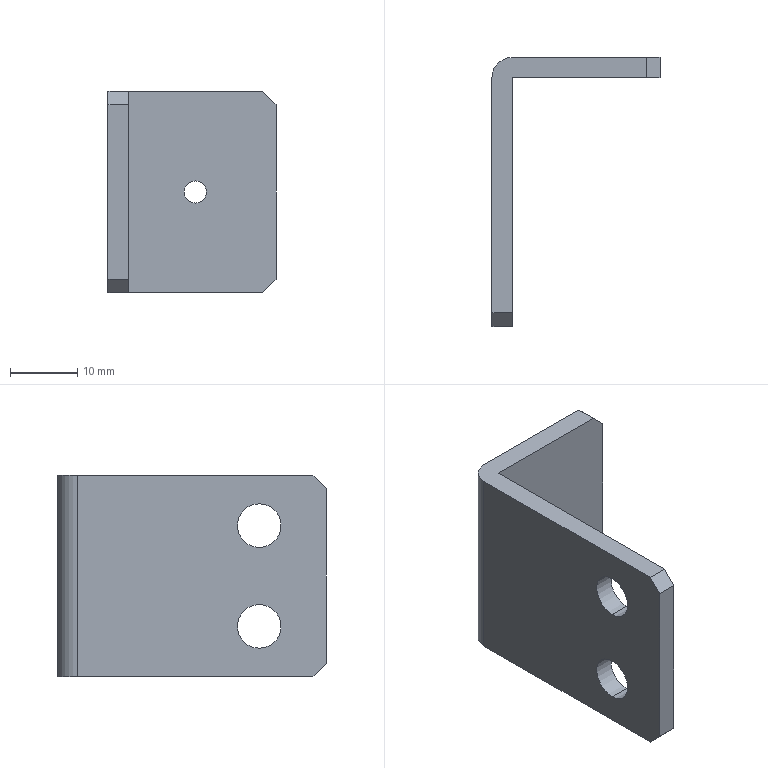Part | STEP file | 0228_210_Bracket | 1 solid | 19 faces | box 25 x 40 x 30 mm | volume 5273 mm3 | plane 12 | cylinder 7 | commonest cylinder face diameters 6.5 x4 3.3 x2 6 x1
STEP:
#1=CARTESIAN_POINT('',(0.,0.,0.));
#2=DIRECTION('',(0.,0.,1.));
#3=DIRECTION('',(1.,0.,0.));
#4=AXIS2_PLACEMENT_3D('',#1,#2,#3);
#5=CARTESIAN_POINT('',(13.,-3.,1.65));
#6=VERTEX_POINT('',#5);
#7=CARTESIAN_POINT('',(13.,0.,1.65));
#8=VERTEX_POINT('',#7);
#9=CARTESIAN_POINT('',(13.,0.,1.65));
#10=DIRECTION('',(0.,1.,0.));
#11=VECTOR('',#10,1.);
#12=LINE('',#9,#11);
#13=CARTESIAN_POINT('',(13.,0.,0.));
#14=DIRECTION('',(0.,1.,0.));
#15=DIRECTION('',(0.,0.,1.));
#16=AXIS2_PLACEMENT_3D('',#13,#14,#15);
#17=CYLINDRICAL_SURFACE('',#16,1.65);
#18=CARTESIAN_POINT('',(6.283,0.));
#19=DIRECTION('',(0.,1.));
#20=VECTOR('',#19,1.);
#21=LINE('',#18,#20);
#22=(GEOMETRIC_REPRESENTATION_CONTEXT(2)PARAMETRIC_REPRESENTATION_CONTEXT()REPRESENTATION_CONTEXT('',''));
#23=DEFINITIONAL_REPRESENTATION('',(#21),#22);
#24=PCURVE('',#17,#23);
#25=CARTESIAN_POINT('',(13.,0.,0.));
#26=DIRECTION('',(0.,1.,0.));
#27=DIRECTION('',(0.,0.,1.));
#28=AXIS2_PLACEMENT_3D('',#25,#26,#27);
#29=CYLINDRICAL_SURFACE('',#28,1.65);
#30=CARTESIAN_POINT('',(0.,0.));
#31=DIRECTION('',(0.,1.));
#32=VECTOR('',#31,1.);
#33=LINE('',#30,#32);
#34=(GEOMETRIC_REPRESENTATION_CONTEXT(2)PARAMETRIC_REPRESENTATION_CONTEXT()REPRESENTATION_CONTEXT('',''));
#35=DEFINITIONAL_REPRESENTATION('',(#33),#34);
#36=PCURVE('',#29,#35);
#37=SURFACE_CURVE('',#12,(#24,#36),.PCURVE_S1.);
#38=EDGE_CURVE('',#6,#8,#37,.T.);
#39=ORIENTED_EDGE('',*,*,#38,.T.);
#40=CARTESIAN_POINT('',(13.,0.,-1.65));
#41=VERTEX_POINT('',#40);
#42=CARTESIAN_POINT('',(13.,0.,0.));
#43=DIRECTION('',(0.,1.,0.));
#44=DIRECTION('',(0.,0.,1.));
#45=AXIS2_PLACEMENT_3D('',#42,#43,#44);
#46=CIRCLE('',#45,1.65);
#47=CARTESIAN_POINT('',(0.,0.));
#48=DIRECTION('',(1.,0.));
#49=VECTOR('',#48,1.);
#50=LINE('',#47,#49);
#51=(GEOMETRIC_REPRESENTATION_CONTEXT(2)PARAMETRIC_REPRESENTATION_CONTEXT()REPRESENTATION_CONTEXT('',''));
#52=DEFINITIONAL_REPRESENTATION('',(#50),#51);
#53=PCURVE('',#17,#52);
#54=CARTESIAN_POINT('',(25.,0.,15.));
#55=DIRECTION('',(0.,-1.,0.));
#56=DIRECTION('',(1.,0.,0.));
#57=AXIS2_PLACEMENT_3D('',#54,#55,#56);
#58=PLANE('',#57);
#59=CARTESIAN_POINT('',(-12.,-13.35));
#60=CARTESIAN_POINT('',(-9.142,-13.35));
#61=CARTESIAN_POINT('',(-10.571,-15.825));
#62=CARTESIAN_POINT('',(-12.,-18.3));
#63=CARTESIAN_POINT('',(-13.429,-15.825));
#64=CARTESIAN_POINT('',(-14.858,-13.35));
#65=CARTESIAN_POINT('',(-12.,-13.35));
#66=(BOUNDED_CURVE()B_SPLINE_CURVE(2,(#59,#60,#61,#62,#63,#64,#65),.UNSPECIFIED.,.T.,.F.)B_SPLINE_CURVE_WITH_KNOTS((1,2,2,2,2,1),(-2.094,0.,2.094,4.189,6.283,8.378),.UNSPECIFIED.)CURVE()GEOMETRIC_REPRESENTATION_ITEM()RATIONAL_B_SPLINE_CURVE((1.,0.5,1.,0.5,1.,0.5,1.))REPRESENTATION_ITEM(''));
#67=(GEOMETRIC_REPRESENTATION_CONTEXT(2)PARAMETRIC_REPRESENTATION_CONTEXT()REPRESENTATION_CONTEXT('',''));
#68=DEFINITIONAL_REPRESENTATION('',(#66),#67);
#69=PCURVE('',#58,#68);
#70=SURFACE_CURVE('',#46,(#53,#69),.PCURVE_S1.);
#71=EDGE_CURVE('',#41,#8,#70,.T.);
#72=ORIENTED_EDGE('',*,*,#71,.F.);
#73=CARTESIAN_POINT('',(13.,-3.,-1.65));
#74=VERTEX_POINT('',#73);
#75=CARTESIAN_POINT('',(13.,0.,-1.65));
#76=DIRECTION('',(0.,1.,0.));
#77=VECTOR('',#76,1.);
#78=LINE('',#75,#77);
#79=CARTESIAN_POINT('',(3.142,0.));
#80=DIRECTION('',(0.,1.));
#81=VECTOR('',#80,1.);
#82=LINE('',#79,#81);
#83=(GEOMETRIC_REPRESENTATION_CONTEXT(2)PARAMETRIC_REPRESENTATION_CONTEXT()REPRESENTATION_CONTEXT('',''));
#84=DEFINITIONAL_REPRESENTATION('',(#82),#83);
#85=PCURVE('',#17,#84);
#86=CARTESIAN_POINT('',(3.142,0.));
#87=DIRECTION('',(0.,1.));
#88=VECTOR('',#87,1.);
#89=LINE('',#86,#88);
#90=(GEOMETRIC_REPRESENTATION_CONTEXT(2)PARAMETRIC_REPRESENTATION_CONTEXT()REPRESENTATION_CONTEXT('',''));
#91=DEFINITIONAL_REPRESENTATION('',(#89),#90);
#92=PCURVE('',#29,#91);
#93=SURFACE_CURVE('',#78,(#85,#92),.PCURVE_S1.);
#94=EDGE_CURVE('',#74,#41,#93,.T.);
#95=ORIENTED_EDGE('',*,*,#94,.F.);
#96=CARTESIAN_POINT('',(13.,-3.,0.));
#97=DIRECTION('',(0.,1.,0.));
#98=DIRECTION('',(-1.,0.,0.));
#99=AXIS2_PLACEMENT_3D('',#96,#97,#98);
#100=CIRCLE('',#99,1.65);
#101=CARTESIAN_POINT('',(-1.571,-3.));
#102=DIRECTION('',(1.,0.));
#103=VECTOR('',#102,1.);
#104=LINE('',#101,#103);
#105=(GEOMETRIC_REPRESENTATION_CONTEXT(2)PARAMETRIC_REPRESENTATION_CONTEXT()REPRESENTATION_CONTEXT('',''));
#106=DEFINITIONAL_REPRESENTATION('',(#104),#105);
#107=PCURVE('',#17,#106);
#108=CARTESIAN_POINT('',(25.,-3.,15.));
#109=DIRECTION('',(0.,1.,0.));
#110=DIRECTION('',(-1.,0.,0.));
#111=AXIS2_PLACEMENT_3D('',#108,#109,#110);
#112=PLANE('',#111);
#113=CARTESIAN_POINT('',(12.,-15.));
#114=DIRECTION('',(1.,0.));
#115=AXIS2_PLACEMENT_2D('',#113,#114);
#116=CIRCLE('',#115,1.65);
#117=(GEOMETRIC_REPRESENTATION_CONTEXT(2)PARAMETRIC_REPRESENTATION_CONTEXT()REPRESENTATION_CONTEXT('',''));
#118=DEFINITIONAL_REPRESENTATION('',(#116),#117);
#119=PCURVE('',#112,#118);
#120=SURFACE_CURVE('',#100,(#107,#119),.PCURVE_S1.);
#121=EDGE_CURVE('',#74,#6,#120,.T.);
#122=ORIENTED_EDGE('',*,*,#121,.T.);
#123=EDGE_LOOP('',(#39,#72,#95,#122));
#124=FACE_BOUND('',#123,.F.);
#125=ADVANCED_FACE('',(#124),#17,.F.);
#126=CARTESIAN_POINT('',(0.,-30.,4.25));
#127=VERTEX_POINT('',#126);
#128=CARTESIAN_POINT('',(3.,-30.,4.25));
#129=VERTEX_POINT('',#128);
#130=CARTESIAN_POINT('',(3.,-30.,4.25));
#131=DIRECTION('',(1.,0.,0.));
#132=VECTOR('',#131,1.);
#133=LINE('',#130,#132);
#134=CARTESIAN_POINT('',(3.,-30.,7.5));
#135=DIRECTION('',(1.,0.,0.));
#136=DIRECTION('',(0.,0.,-1.));
#137=AXIS2_PLACEMENT_3D('',#134,#135,#136);
#138=CYLINDRICAL_SURFACE('',#137,3.25);
#139=CARTESIAN_POINT('',(6.283,0.));
#140=DIRECTION('',(0.,1.));
#141=VECTOR('',#140,1.);
#142=LINE('',#139,#141);
#143=(GEOMETRIC_REPRESENTATION_CONTEXT(2)PARAMETRIC_REPRESENTATION_CONTEXT()REPRESENTATION_CONTEXT('',''));
#144=DEFINITIONAL_REPRESENTATION('',(#142),#143);
#145=PCURVE('',#138,#144);
#146=CARTESIAN_POINT('',(3.,-30.,7.5));
#147=DIRECTION('',(1.,0.,0.));
#148=DIRECTION('',(0.,0.,-1.));
#149=AXIS2_PLACEMENT_3D('',#146,#147,#148);
#150=CYLINDRICAL_SURFACE('',#149,3.25);
#151=CARTESIAN_POINT('',(0.,0.));
#152=DIRECTION('',(0.,1.));
#153=VECTOR('',#152,1.);
#154=LINE('',#151,#153);
#155=(GEOMETRIC_REPRESENTATION_CONTEXT(2)PARAMETRIC_REPRESENTATION_CONTEXT()REPRESENTATION_CONTEXT('',''));
#156=DEFINITIONAL_REPRESENTATION('',(#154),#155);
#157=PCURVE('',#150,#156);
#158=SURFACE_CURVE('',#133,(#145,#157),.PCURVE_S1.);
#159=EDGE_CURVE('',#127,#129,#158,.T.);
#160=ORIENTED_EDGE('',*,*,#159,.T.);
#161=CARTESIAN_POINT('',(3.,-30.,10.75));
#162=VERTEX_POINT('',#161);
#163=CARTESIAN_POINT('',(3.,-30.,7.5));
#164=DIRECTION('',(1.,0.,0.));
#165=DIRECTION('',(0.,0.,-1.));
#166=AXIS2_PLACEMENT_3D('',#163,#164,#165);
#167=CIRCLE('',#166,3.25);
#168=CARTESIAN_POINT('',(0.,0.));
#169=DIRECTION('',(1.,0.));
#170=VECTOR('',#169,1.);
#171=LINE('',#168,#170);
#172=(GEOMETRIC_REPRESENTATION_CONTEXT(2)PARAMETRIC_REPRESENTATION_CONTEXT()REPRESENTATION_CONTEXT('',''));
#173=DEFINITIONAL_REPRESENTATION('',(#171),#172);
#174=PCURVE('',#138,#173);
#175=CARTESIAN_POINT('',(3.,-3.,15.));
#176=DIRECTION('',(-1.,0.,0.));
#177=DIRECTION('',(0.,-1.,0.));
#178=AXIS2_PLACEMENT_3D('',#175,#176,#177);
#179=PLANE('',#178);
#180=CARTESIAN_POINT('',(27.,-10.75));
#181=CARTESIAN_POINT('',(21.371,-10.75));
#182=CARTESIAN_POINT('',(24.185,-5.875));
#183=CARTESIAN_POINT('',(27.,-1.));
#184=CARTESIAN_POINT('',(29.815,-5.875));
#185=CARTESIAN_POINT('',(32.629,-10.75));
#186=CARTESIAN_POINT('',(27.,-10.75));
#187=(BOUNDED_CURVE()B_SPLINE_CURVE(2,(#180,#181,#182,#183,#184,#185,#186),.UNSPECIFIED.,.T.,.F.)B_SPLINE_CURVE_WITH_KNOTS((1,2,2,2,2,1),(-2.094,0.,2.094,4.189,6.283,8.378),.UNSPECIFIED.)CURVE()GEOMETRIC_REPRESENTATION_ITEM()RATIONAL_B_SPLINE_CURVE((1.,0.5,1.,0.5,1.,0.5,1.))REPRESENTATION_ITEM(''));
#188=(GEOMETRIC_REPRESENTATION_CONTEXT(2)PARAMETRIC_REPRESENTATION_CONTEXT()REPRESENTATION_CONTEXT('',''));
#189=DEFINITIONAL_REPRESENTATION('',(#187),#188);
#190=PCURVE('',#179,#189);
#191=SURFACE_CURVE('',#167,(#174,#190),.PCURVE_S1.);
#192=EDGE_CURVE('',#162,#129,#191,.T.);
#193=ORIENTED_EDGE('',*,*,#192,.F.);
#194=CARTESIAN_POINT('',(0.,-30.,10.75));
#195=VERTEX_POINT('',#194);
#196=CARTESIAN_POINT('',(3.,-30.,10.75));
#197=DIRECTION('',(1.,0.,0.));
#198=VECTOR('',#197,1.);
#199=LINE('',#196,#198);
#200=CARTESIAN_POINT('',(3.142,0.));
#201=DIRECTION('',(0.,1.));
#202=VECTOR('',#201,1.);
#203=LINE('',#200,#202);
#204=(GEOMETRIC_REPRESENTATION_CONTEXT(2)PARAMETRIC_REPRESENTATION_CONTEXT()REPRESENTATION_CONTEXT('',''));
#205=DEFINITIONAL_REPRESENTATION('',(#203),#204);
#206=PCURVE('',#138,#205);
#207=CARTESIAN_POINT('',(3.142,0.));
#208=DIRECTION('',(0.,1.));
#209=VECTOR('',#208,1.);
#210=LINE('',#207,#209);
#211=(GEOMETRIC_REPRESENTATION_CONTEXT(2)PARAMETRIC_REPRESENTATION_CONTEXT()REPRESENTATION_CONTEXT('',''));
#212=DEFINITIONAL_REPRESENTATION('',(#210),#211);
#213=PCURVE('',#150,#212);
#214=SURFACE_CURVE('',#199,(#206,#213),.PCURVE_S1.);
#215=EDGE_CURVE('',#195,#162,#214,.T.);
#216=ORIENTED_EDGE('',*,*,#215,.F.);
#217=CARTESIAN_POINT('',(0.,-30.,7.5));
#218=DIRECTION('',(1.,0.,0.));
#219=DIRECTION('',(0.,0.,-1.));
#220=AXIS2_PLACEMENT_3D('',#217,#218,#219);
#221=CIRCLE('',#220,3.25);
#222=CARTESIAN_POINT('',(0.,-3.));
#223=DIRECTION('',(1.,0.));
#224=VECTOR('',#223,1.);
#225=LINE('',#222,#224);
#226=(GEOMETRIC_REPRESENTATION_CONTEXT(2)PARAMETRIC_REPRESENTATION_CONTEXT()REPRESENTATION_CONTEXT('',''));
#227=DEFINITIONAL_REPRESENTATION('',(#225),#226);
#228=PCURVE('',#138,#227);
#229=CARTESIAN_POINT('',(0.,0.,15.));
#230=DIRECTION('',(1.,0.,0.));
#231=DIRECTION('',(0.,1.,0.));
#232=AXIS2_PLACEMENT_3D('',#229,#230,#231);
#233=PLANE('',#232);
#234=CARTESIAN_POINT('',(-30.,-7.5));
#235=DIRECTION('',(0.,-1.));
#236=AXIS2_PLACEMENT_2D('',#234,#235);
#237=CIRCLE('',#236,3.25);
#238=(GEOMETRIC_REPRESENTATION_CONTEXT(2)PARAMETRIC_REPRESENTATION_CONTEXT()REPRESENTATION_CONTEXT('',''));
#239=DEFINITIONAL_REPRESENTATION('',(#237),#238);
#240=PCURVE('',#233,#239);
#241=SURFACE_CURVE('',#221,(#228,#240),.PCURVE_S1.);
#242=EDGE_CURVE('',#195,#127,#241,.T.);
#243=ORIENTED_EDGE('',*,*,#242,.T.);
#244=EDGE_LOOP('',(#160,#193,#216,#243));
#245=FACE_BOUND('',#244,.F.);
#246=ADVANCED_FACE('',(#245),#138,.F.);
#247=CARTESIAN_POINT('',(0.,-30.,-10.75));
#248=VERTEX_POINT('',#247);
#249=CARTESIAN_POINT('',(3.,-30.,-10.75));
#250=VERTEX_POINT('',#249);
#251=CARTESIAN_POINT('',(3.,-30.,-10.75));
#252=DIRECTION('',(1.,0.,0.));
#253=VECTOR('',#252,1.);
#254=LINE('',#251,#253);
#255=CARTESIAN_POINT('',(3.,-30.,-7.5));
#256=DIRECTION('',(1.,0.,0.));
#257=DIRECTION('',(0.,0.,-1.));
#258=AXIS2_PLACEMENT_3D('',#255,#256,#257);
#259=CYLINDRICAL_SURFACE('',#258,3.25);
#260=CARTESIAN_POINT('',(6.283,0.));
#261=DIRECTION('',(0.,1.));
#262=VECTOR('',#261,1.);
#263=LINE('',#260,#262);
#264=(GEOMETRIC_REPRESENTATION_CONTEXT(2)PARAMETRIC_REPRESENTATION_CONTEXT()REPRESENTATION_CONTEXT('',''));
#265=DEFINITIONAL_REPRESENTATION('',(#263),#264);
#266=PCURVE('',#259,#265);
#267=CARTESIAN_POINT('',(3.,-30.,-7.5));
#268=DIRECTION('',(1.,0.,0.));
#269=DIRECTION('',(0.,0.,-1.));
#270=AXIS2_PLACEMENT_3D('',#267,#268,#269);
#271=CYLINDRICAL_SURFACE('',#270,3.25);
#272=CARTESIAN_POINT('',(0.,0.));
#273=DIRECTION('',(0.,1.));
#274=VECTOR('',#273,1.);
#275=LINE('',#272,#274);
#276=(GEOMETRIC_REPRESENTATION_CONTEXT(2)PARAMETRIC_REPRESENTATION_CONTEXT()REPRESENTATION_CONTEXT('',''));
#277=DEFINITIONAL_REPRESENTATION('',(#275),#276);
#278=PCURVE('',#271,#277);
#279=SURFACE_CURVE('',#254,(#266,#278),.PCURVE_S1.);
#280=EDGE_CURVE('',#248,#250,#279,.T.);
#281=ORIENTED_EDGE('',*,*,#280,.T.);
#282=CARTESIAN_POINT('',(3.,-30.,-4.25));
#283=VERTEX_POINT('',#282);
#284=CARTESIAN_POINT('',(3.,-30.,-7.5));
#285=DIRECTION('',(1.,0.,0.));
#286=DIRECTION('',(0.,0.,-1.));
#287=AXIS2_PLACEMENT_3D('',#284,#285,#286);
#288=CIRCLE('',#287,3.25);
#289=CARTESIAN_POINT('',(0.,0.));
#290=DIRECTION('',(1.,0.));
#291=VECTOR('',#290,1.);
#292=LINE('',#289,#291);
#293=(GEOMETRIC_REPRESENTATION_CONTEXT(2)PARAMETRIC_REPRESENTATION_CONTEXT()REPRESENTATION_CONTEXT('',''));
#294=DEFINITIONAL_REPRESENTATION('',(#292),#293);
#295=PCURVE('',#259,#294);
#296=CARTESIAN_POINT('',(27.,-25.75));
#297=CARTESIAN_POINT('',(21.371,-25.75));
#298=CARTESIAN_POINT('',(24.185,-20.875));
#299=CARTESIAN_POINT('',(27.,-16.));
#300=CARTESIAN_POINT('',(29.815,-20.875));
#301=CARTESIAN_POINT('',(32.629,-25.75));
#302=CARTESIAN_POINT('',(27.,-25.75));
#303=(BOUNDED_CURVE()B_SPLINE_CURVE(2,(#296,#297,#298,#299,#300,#301,#302),.UNSPECIFIED.,.T.,.F.)B_SPLINE_CURVE_WITH_KNOTS((1,2,2,2,2,1),(-2.094,0.,2.094,4.189,6.283,8.378),.UNSPECIFIED.)CURVE()GEOMETRIC_REPRESENTATION_ITEM()RATIONAL_B_SPLINE_CURVE((1.,0.5,1.,0.5,1.,0.5,1.))REPRESENTATION_ITEM(''));
#304=(GEOMETRIC_REPRESENTATION_CONTEXT(2)PARAMETRIC_REPRESENTATION_CONTEXT()REPRESENTATION_CONTEXT('',''));
#305=DEFINITIONAL_REPRESENTATION('',(#303),#304);
#306=PCURVE('',#179,#305);
#307=SURFACE_CURVE('',#288,(#295,#306),.PCURVE_S1.);
#308=EDGE_CURVE('',#283,#250,#307,.T.);
#309=ORIENTED_EDGE('',*,*,#308,.F.);
#310=CARTESIAN_POINT('',(0.,-30.,-4.25));
#311=VERTEX_POINT('',#310);
#312=CARTESIAN_POINT('',(3.,-30.,-4.25));
#313=DIRECTION('',(1.,0.,0.));
#314=VECTOR('',#313,1.);
#315=LINE('',#312,#314);
#316=CARTESIAN_POINT('',(3.142,0.));
#317=DIRECTION('',(0.,1.));
#318=VECTOR('',#317,1.);
#319=LINE('',#316,#318);
#320=(GEOMETRIC_REPRESENTATION_CONTEXT(2)PARAMETRIC_REPRESENTATION_CONTEXT()REPRESENTATION_CONTEXT('',''));
#321=DEFINITIONAL_REPRESENTATION('',(#319),#320);
#322=PCURVE('',#259,#321);
#323=CARTESIAN_POINT('',(3.142,0.));
#324=DIRECTION('',(0.,1.));
#325=VECTOR('',#324,1.);
#326=LINE('',#323,#325);
#327=(GEOMETRIC_REPRESENTATION_CONTEXT(2)PARAMETRIC_REPRESENTATION_CONTEXT()REPRESENTATION_CONTEXT('',''));
#328=DEFINITIONAL_REPRESENTATION('',(#326),#327);
#329=PCURVE('',#271,#328);
#330=SURFACE_CURVE('',#315,(#322,#329),.PCURVE_S1.);
#331=EDGE_CURVE('',#311,#283,#330,.T.);
#332=ORIENTED_EDGE('',*,*,#331,.F.);
#333=CARTESIAN_POINT('',(0.,-30.,-7.5));
#334=DIRECTION('',(1.,0.,0.));
#335=DIRECTION('',(0.,0.,-1.));
#336=AXIS2_PLACEMENT_3D('',#333,#334,#335);
#337=CIRCLE('',#336,3.25);
#338=CARTESIAN_POINT('',(0.,-3.));
#339=DIRECTION('',(1.,0.));
#340=VECTOR('',#339,1.);
#341=LINE('',#338,#340);
#342=(GEOMETRIC_REPRESENTATION_CONTEXT(2)PARAMETRIC_REPRESENTATION_CONTEXT()REPRESENTATION_CONTEXT('',''));
#343=DEFINITIONAL_REPRESENTATION('',(#341),#342);
#344=PCURVE('',#259,#343);
#345=CARTESIAN_POINT('',(-30.,-22.5));
#346=DIRECTION('',(0.,-1.));
#347=AXIS2_PLACEMENT_2D('',#345,#346);
#348=CIRCLE('',#347,3.25);
#349=(GEOMETRIC_REPRESENTATION_CONTEXT(2)PARAMETRIC_REPRESENTATION_CONTEXT()REPRESENTATION_CONTEXT('',''));
#350=DEFINITIONAL_REPRESENTATION('',(#348),#349);
#351=PCURVE('',#233,#350);
#352=SURFACE_CURVE('',#337,(#344,#351),.PCURVE_S1.);
#353=EDGE_CURVE('',#311,#248,#352,.T.);
#354=ORIENTED_EDGE('',*,*,#353,.T.);
#355=EDGE_LOOP('',(#281,#309,#332,#354));
#356=FACE_BOUND('',#355,.F.);
#357=ADVANCED_FACE('',(#356),#259,.F.);
#358=CARTESIAN_POINT('',(25.,-3.,13.));
#359=VERTEX_POINT('',#358);
#360=CARTESIAN_POINT('',(25.,-3.,-13.));
#361=VERTEX_POINT('',#360);
#362=CARTESIAN_POINT('',(25.,-3.,15.));
#363=DIRECTION('',(0.,0.,-1.));
#364=VECTOR('',#363,1.);
#365=LINE('',#362,#364);
#366=CARTESIAN_POINT('',(25.,0.,15.));
#367=DIRECTION('',(-1.,0.,0.));
#368=DIRECTION('',(0.,0.,1.));
#369=AXIS2_PLACEMENT_3D('',#366,#367,#368);
#370=PLANE('',#369);
#371=CARTESIAN_POINT('',(0.,-3.));
#372=DIRECTION('',(-1.,0.));
#373=VECTOR('',#372,1.);
#374=LINE('',#371,#373);
#375=(GEOMETRIC_REPRESENTATION_CONTEXT(2)PARAMETRIC_REPRESENTATION_CONTEXT()REPRESENTATION_CONTEXT('',''));
#376=DEFINITIONAL_REPRESENTATION('',(#374),#375);
#377=PCURVE('',#370,#376);
#378=CARTESIAN_POINT('',(0.,0.));
#379=DIRECTION('',(0.,-1.));
#380=VECTOR('',#379,1.);
#381=LINE('',#378,#380);
#382=(GEOMETRIC_REPRESENTATION_CONTEXT(2)PARAMETRIC_REPRESENTATION_CONTEXT()REPRESENTATION_CONTEXT('',''));
#383=DEFINITIONAL_REPRESENTATION('',(#381),#382);
#384=PCURVE('',#112,#383);
#385=SURFACE_CURVE('',#365,(#377,#384),.PCURVE_S1.);
#386=EDGE_CURVE('',#359,#361,#385,.T.);
#387=ORIENTED_EDGE('',*,*,#386,.T.);
#388=CARTESIAN_POINT('',(25.,0.,-13.));
#389=VERTEX_POINT('',#388);
#390=CARTESIAN_POINT('',(25.,0.,-13.));
#391=DIRECTION('',(0.,1.,0.));
#392=VECTOR('',#391,1.);
#393=LINE('',#390,#392);
#394=CARTESIAN_POINT('',(-28.,0.));
#395=DIRECTION('',(0.,1.));
#396=VECTOR('',#395,1.);
#397=LINE('',#394,#396);
#398=(GEOMETRIC_REPRESENTATION_CONTEXT(2)PARAMETRIC_REPRESENTATION_CONTEXT()REPRESENTATION_CONTEXT('',''));
#399=DEFINITIONAL_REPRESENTATION('',(#397),#398);
#400=PCURVE('',#370,#399);
#401=CARTESIAN_POINT('',(25.,0.,-13.));
#402=DIRECTION('',(0.7071,0.,-0.7071));
#403=DIRECTION('',(-0.7071,0.,-0.7071));
#404=AXIS2_PLACEMENT_3D('',#401,#402,#403);
#405=PLANE('',#404);
#406=CARTESIAN_POINT('',(0.,0.));
#407=DIRECTION('',(0.,1.));
#408=VECTOR('',#407,1.);
#409=LINE('',#406,#408);
#410=(GEOMETRIC_REPRESENTATION_CONTEXT(2)PARAMETRIC_REPRESENTATION_CONTEXT()REPRESENTATION_CONTEXT('',''));
#411=DEFINITIONAL_REPRESENTATION('',(#409),#410);
#412=PCURVE('',#405,#411);
#413=SURFACE_CURVE('',#393,(#400,#412),.PCURVE_S1.);
#414=EDGE_CURVE('',#361,#389,#413,.T.);
#415=ORIENTED_EDGE('',*,*,#414,.T.);
#416=CARTESIAN_POINT('',(25.,0.,13.));
#417=VERTEX_POINT('',#416);
#418=CARTESIAN_POINT('',(25.,0.,15.));
#419=DIRECTION('',(0.,0.,-1.));
#420=VECTOR('',#419,1.);
#421=LINE('',#418,#420);
#422=CARTESIAN_POINT('',(0.,0.));
#423=DIRECTION('',(-1.,0.));
#424=VECTOR('',#423,1.);
#425=LINE('',#422,#424);
#426=(GEOMETRIC_REPRESENTATION_CONTEXT(2)PARAMETRIC_REPRESENTATION_CONTEXT()REPRESENTATION_CONTEXT('',''));
#427=DEFINITIONAL_REPRESENTATION('',(#425),#426);
#428=PCURVE('',#370,#427);
#429=CARTESIAN_POINT('',(0.,0.));
#430=DIRECTION('',(0.,-1.));
#431=VECTOR('',#430,1.);
#432=LINE('',#429,#431);
#433=(GEOMETRIC_REPRESENTATION_CONTEXT(2)PARAMETRIC_REPRESENTATION_CONTEXT()REPRESENTATION_CONTEXT('',''));
#434=DEFINITIONAL_REPRESENTATION('',(#432),#433);
#435=PCURVE('',#58,#434);
#436=SURFACE_CURVE('',#421,(#428,#435),.PCURVE_S1.);
#437=EDGE_CURVE('',#417,#389,#436,.T.);
#438=ORIENTED_EDGE('',*,*,#437,.F.);
#439=CARTESIAN_POINT('',(25.,0.,13.));
#440=DIRECTION('',(0.,-1.,0.));
#441=VECTOR('',#440,1.);
#442=LINE('',#439,#441);
#443=CARTESIAN_POINT('',(-2.,0.));
#444=DIRECTION('',(0.,-1.));
#445=VECTOR('',#444,1.);
#446=LINE('',#443,#445);
#447=(GEOMETRIC_REPRESENTATION_CONTEXT(2)PARAMETRIC_REPRESENTATION_CONTEXT()REPRESENTATION_CONTEXT('',''));
#448=DEFINITIONAL_REPRESENTATION('',(#446),#447);
#449=PCURVE('',#370,#448);
#450=CARTESIAN_POINT('',(23.,-3.,15.));
#451=DIRECTION('',(-0.7071,0.,-0.7071));
#452=DIRECTION('',(-0.7071,0.,0.7071));
#453=AXIS2_PLACEMENT_3D('',#450,#451,#452);
#454=PLANE('',#453);
#455=CARTESIAN_POINT('',(-2.828,3.));
#456=DIRECTION('',(0.,-1.));
#457=VECTOR('',#456,1.);
#458=LINE('',#455,#457);
#459=(GEOMETRIC_REPRESENTATION_CONTEXT(2)PARAMETRIC_REPRESENTATION_CONTEXT()REPRESENTATION_CONTEXT('',''));
#460=DEFINITIONAL_REPRESENTATION('',(#458),#459);
#461=PCURVE('',#454,#460);
#462=SURFACE_CURVE('',#442,(#449,#461),.PCURVE_S1.);
#463=EDGE_CURVE('',#417,#359,#462,.T.);
#464=ORIENTED_EDGE('',*,*,#463,.T.);
#465=EDGE_LOOP('',(#387,#415,#438,#464));
#466=FACE_BOUND('',#465,.T.);
#467=ADVANCED_FACE('',(#466),#370,.F.);
#468=CARTESIAN_POINT('',(13.,0.,0.));
#469=DIRECTION('',(0.,1.,0.));
#470=DIRECTION('',(0.,0.,1.));
#471=AXIS2_PLACEMENT_3D('',#468,#469,#470);
#472=CIRCLE('',#471,1.65);
#473=CARTESIAN_POINT('',(-12.,-13.35));
#474=CARTESIAN_POINT('',(-9.142,-13.35));
#475=CARTESIAN_POINT('',(-10.571,-15.825));
#476=CARTESIAN_POINT('',(-12.,-18.3));
#477=CARTESIAN_POINT('',(-13.429,-15.825));
#478=CARTESIAN_POINT('',(-14.858,-13.35));
#479=CARTESIAN_POINT('',(-12.,-13.35));
#480=(BOUNDED_CURVE()B_SPLINE_CURVE(2,(#473,#474,#475,#476,#477,#478,#479),.UNSPECIFIED.,.T.,.F.)B_SPLINE_CURVE_WITH_KNOTS((1,2,2,2,2,1),(-2.094,0.,2.094,4.189,6.283,8.378),.UNSPECIFIED.)CURVE()GEOMETRIC_REPRESENTATION_ITEM()RATIONAL_B_SPLINE_CURVE((1.,0.5,1.,0.5,1.,0.5,1.))REPRESENTATION_ITEM(''));
#481=(GEOMETRIC_REPRESENTATION_CONTEXT(2)PARAMETRIC_REPRESENTATION_CONTEXT()REPRESENTATION_CONTEXT('',''));
#482=DEFINITIONAL_REPRESENTATION('',(#480),#481);
#483=PCURVE('',#58,#482);
#484=CARTESIAN_POINT('',(0.,0.));
#485=DIRECTION('',(1.,0.));
#486=VECTOR('',#485,1.);
#487=LINE('',#484,#486);
#488=(GEOMETRIC_REPRESENTATION_CONTEXT(2)PARAMETRIC_REPRESENTATION_CONTEXT()REPRESENTATION_CONTEXT('',''));
#489=DEFINITIONAL_REPRESENTATION('',(#487),#488);
#490=PCURVE('',#29,#489);
#491=SURFACE_CURVE('',#472,(#483,#490),.PCURVE_S1.);
#492=EDGE_CURVE('',#8,#41,#491,.T.);
#493=ORIENTED_EDGE('',*,*,#492,.F.);
#494=ORIENTED_EDGE('',*,*,#71,.F.);
#495=EDGE_LOOP('',(#493,#494));
#496=FACE_BOUND('',#495,.T.);
#497=ORIENTED_EDGE('',*,*,#437,.T.);
#498=CARTESIAN_POINT('',(23.,0.,-15.));
#499=VERTEX_POINT('',#498);
#500=CARTESIAN_POINT('',(25.,0.,-13.));
#501=DIRECTION('',(-0.7071,0.,-0.7071));
#502=VECTOR('',#501,1.);
#503=LINE('',#500,#502);
#504=CARTESIAN_POINT('',(0.,-28.));
#505=DIRECTION('',(-0.7071,-0.7071));
#506=VECTOR('',#505,1.);
#507=LINE('',#504,#506);
#508=(GEOMETRIC_REPRESENTATION_CONTEXT(2)PARAMETRIC_REPRESENTATION_CONTEXT()REPRESENTATION_CONTEXT('',''));
#509=DEFINITIONAL_REPRESENTATION('',(#507),#508);
#510=PCURVE('',#58,#509);
#511=CARTESIAN_POINT('',(0.,0.));
#512=DIRECTION('',(1.,0.));
#513=VECTOR('',#512,1.);
#514=LINE('',#511,#513);
#515=(GEOMETRIC_REPRESENTATION_CONTEXT(2)PARAMETRIC_REPRESENTATION_CONTEXT()REPRESENTATION_CONTEXT('',''));
#516=DEFINITIONAL_REPRESENTATION('',(#514),#515);
#517=PCURVE('',#405,#516);
#518=SURFACE_CURVE('',#503,(#510,#517),.PCURVE_S1.);
#519=EDGE_CURVE('',#389,#499,#518,.T.);
#520=ORIENTED_EDGE('',*,*,#519,.T.);
#521=CARTESIAN_POINT('',(3.,0.,-15.));
#522=VERTEX_POINT('',#521);
#523=CARTESIAN_POINT('',(25.,0.,-15.));
#524=DIRECTION('',(-1.,0.,0.));
#525=VECTOR('',#524,1.);
#526=LINE('',#523,#525);
#527=CARTESIAN_POINT('',(0.,-30.));
#528=DIRECTION('',(-1.,0.));
#529=VECTOR('',#528,1.);
#530=LINE('',#527,#529);
#531=(GEOMETRIC_REPRESENTATION_CONTEXT(2)PARAMETRIC_REPRESENTATION_CONTEXT()REPRESENTATION_CONTEXT('',''));
#532=DEFINITIONAL_REPRESENTATION('',(#530),#531);
#533=PCURVE('',#58,#532);
#534=CARTESIAN_POINT('',(25.,-3.,-15.));
#535=DIRECTION('',(0.,0.,-1.));
#536=DIRECTION('',(-1.,0.,0.));
#537=AXIS2_PLACEMENT_3D('',#534,#535,#536);
#538=PLANE('',#537);
#539=CARTESIAN_POINT('',(0.,3.));
#540=DIRECTION('',(1.,0.));
#541=VECTOR('',#540,1.);
#542=LINE('',#539,#541);
#543=(GEOMETRIC_REPRESENTATION_CONTEXT(2)PARAMETRIC_REPRESENTATION_CONTEXT()REPRESENTATION_CONTEXT('',''));
#544=DEFINITIONAL_REPRESENTATION('',(#542),#543);
#545=PCURVE('',#538,#544);
#546=SURFACE_CURVE('',#526,(#533,#545),.PCURVE_S1.);
#547=EDGE_CURVE('',#499,#522,#546,.T.);
#548=ORIENTED_EDGE('',*,*,#547,.T.);
#549=CARTESIAN_POINT('',(3.,0.,15.));
#550=VERTEX_POINT('',#549);
#551=CARTESIAN_POINT('',(3.,0.,15.));
#552=DIRECTION('',(0.,0.,1.));
#553=VECTOR('',#552,1.);
#554=LINE('',#551,#553);
#555=CARTESIAN_POINT('',(-22.,0.));
#556=DIRECTION('',(0.,1.));
#557=VECTOR('',#556,1.);
#558=LINE('',#555,#557);
#559=(GEOMETRIC_REPRESENTATION_CONTEXT(2)PARAMETRIC_REPRESENTATION_CONTEXT()REPRESENTATION_CONTEXT('',''));
#560=DEFINITIONAL_REPRESENTATION('',(#558),#559);
#561=PCURVE('',#58,#560);
#562=CARTESIAN_POINT('',(3.,-3.,15.));
#563=DIRECTION('',(0.,0.,-1.));
#564=DIRECTION('',(-1.,0.,0.));
#565=AXIS2_PLACEMENT_3D('',#562,#563,#564);
#566=CYLINDRICAL_SURFACE('',#565,3.);
#567=CARTESIAN_POINT('',(1.571,0.));
#568=DIRECTION('',(0.,-1.));
#569=VECTOR('',#568,1.);
#570=LINE('',#567,#569);
#571=(GEOMETRIC_REPRESENTATION_CONTEXT(2)PARAMETRIC_REPRESENTATION_CONTEXT()REPRESENTATION_CONTEXT('',''));
#572=DEFINITIONAL_REPRESENTATION('',(#570),#571);
#573=PCURVE('',#566,#572);
#574=SURFACE_CURVE('',#554,(#561,#573),.PCURVE_S1.);
#575=EDGE_CURVE('',#522,#550,#574,.T.);
#576=ORIENTED_EDGE('',*,*,#575,.T.);
#577=CARTESIAN_POINT('',(23.,0.,15.));
#578=VERTEX_POINT('',#577);
#579=CARTESIAN_POINT('',(25.,0.,15.));
#580=DIRECTION('',(-1.,0.,0.));
#581=VECTOR('',#580,1.);
#582=LINE('',#579,#581);
#583=CARTESIAN_POINT('',(0.,0.));
#584=DIRECTION('',(-1.,0.));
#585=VECTOR('',#584,1.);
#586=LINE('',#583,#585);
#587=(GEOMETRIC_REPRESENTATION_CONTEXT(2)PARAMETRIC_REPRESENTATION_CONTEXT()REPRESENTATION_CONTEXT('',''));
#588=DEFINITIONAL_REPRESENTATION('',(#586),#587);
#589=PCURVE('',#58,#588);
#590=CARTESIAN_POINT('',(25.,-3.,15.));
#591=DIRECTION('',(0.,0.,-1.));
#592=DIRECTION('',(-1.,0.,0.));
#593=AXIS2_PLACEMENT_3D('',#590,#591,#592);
#594=PLANE('',#593);
#595=CARTESIAN_POINT('',(0.,3.));
#596=DIRECTION('',(1.,0.));
#597=VECTOR('',#596,1.);
#598=LINE('',#595,#597);
#599=(GEOMETRIC_REPRESENTATION_CONTEXT(2)PARAMETRIC_REPRESENTATION_CONTEXT()REPRESENTATION_CONTEXT('',''));
#600=DEFINITIONAL_REPRESENTATION('',(#598),#599);
#601=PCURVE('',#594,#600);
#602=SURFACE_CURVE('',#582,(#589,#601),.PCURVE_S1.);
#603=EDGE_CURVE('',#578,#550,#602,.T.);
#604=ORIENTED_EDGE('',*,*,#603,.F.);
#605=CARTESIAN_POINT('',(23.,0.,15.));
#606=DIRECTION('',(0.7071,0.,-0.7071));
#607=VECTOR('',#606,1.);
#608=LINE('',#605,#607);
#609=CARTESIAN_POINT('',(-2.,0.));
#610=DIRECTION('',(0.7071,-0.7071));
#611=VECTOR('',#610,1.);
#612=LINE('',#609,#611);
#613=(GEOMETRIC_REPRESENTATION_CONTEXT(2)PARAMETRIC_REPRESENTATION_CONTEXT()REPRESENTATION_CONTEXT('',''));
#614=DEFINITIONAL_REPRESENTATION('',(#612),#613);
#615=PCURVE('',#58,#614);
#616=CARTESIAN_POINT('',(0.,3.));
#617=DIRECTION('',(-1.,0.));
#618=VECTOR('',#617,1.);
#619=LINE('',#616,#618);
#620=(GEOMETRIC_REPRESENTATION_CONTEXT(2)PARAMETRIC_REPRESENTATION_CONTEXT()REPRESENTATION_CONTEXT('',''));
#621=DEFINITIONAL_REPRESENTATION('',(#619),#620);
#622=PCURVE('',#454,#621);
#623=SURFACE_CURVE('',#608,(#615,#622),.PCURVE_S1.);
#624=EDGE_CURVE('',#578,#417,#623,.T.);
#625=ORIENTED_EDGE('',*,*,#624,.T.);
#626=EDGE_LOOP('',(#497,#520,#548,#576,#604,#625));
#627=FACE_BOUND('',#626,.T.);
#628=ADVANCED_FACE('',(#496,#627),#58,.F.);
#629=CARTESIAN_POINT('',(0.,-30.,7.5));
#630=DIRECTION('',(1.,0.,0.));
#631=DIRECTION('',(0.,0.,-1.));
#632=AXIS2_PLACEMENT_3D('',#629,#630,#631);
#633=CIRCLE('',#632,3.25);
#634=CARTESIAN_POINT('',(-30.,-7.5));
#635=DIRECTION('',(0.,-1.));
#636=AXIS2_PLACEMENT_2D('',#634,#635);
#637=CIRCLE('',#636,3.25);
#638=(GEOMETRIC_REPRESENTATION_CONTEXT(2)PARAMETRIC_REPRESENTATION_CONTEXT()REPRESENTATION_CONTEXT('',''));
#639=DEFINITIONAL_REPRESENTATION('',(#637),#638);
#640=PCURVE('',#233,#639);
#641=CARTESIAN_POINT('',(0.,-3.));
#642=DIRECTION('',(1.,0.));
#643=VECTOR('',#642,1.);
#644=LINE('',#641,#643);
#645=(GEOMETRIC_REPRESENTATION_CONTEXT(2)PARAMETRIC_REPRESENTATION_CONTEXT()REPRESENTATION_CONTEXT('',''));
#646=DEFINITIONAL_REPRESENTATION('',(#644),#645);
#647=PCURVE('',#150,#646);
#648=SURFACE_CURVE('',#633,(#640,#647),.PCURVE_S1.);
#649=EDGE_CURVE('',#127,#195,#648,.T.);
#650=ORIENTED_EDGE('',*,*,#649,.T.);
#651=ORIENTED_EDGE('',*,*,#242,.T.);
#652=EDGE_LOOP('',(#650,#651));
#653=FACE_BOUND('',#652,.T.);
#654=CARTESIAN_POINT('',(0.,-30.,-7.5));
#655=DIRECTION('',(1.,0.,0.));
#656=DIRECTION('',(0.,0.,-1.));
#657=AXIS2_PLACEMENT_3D('',#654,#655,#656);
#658=CIRCLE('',#657,3.25);
#659=CARTESIAN_POINT('',(-30.,-22.5));
#660=DIRECTION('',(0.,-1.));
#661=AXIS2_PLACEMENT_2D('',#659,#660);
#662=CIRCLE('',#661,3.25);
#663=(GEOMETRIC_REPRESENTATION_CONTEXT(2)PARAMETRIC_REPRESENTATION_CONTEXT()REPRESENTATION_CONTEXT('',''));
#664=DEFINITIONAL_REPRESENTATION('',(#662),#663);
#665=PCURVE('',#233,#664);
#666=CARTESIAN_POINT('',(0.,-3.));
#667=DIRECTION('',(1.,0.));
#668=VECTOR('',#667,1.);
#669=LINE('',#666,#668);
#670=(GEOMETRIC_REPRESENTATION_CONTEXT(2)PARAMETRIC_REPRESENTATION_CONTEXT()REPRESENTATION_CONTEXT('',''));
#671=DEFINITIONAL_REPRESENTATION('',(#669),#670);
#672=PCURVE('',#271,#671);
#673=SURFACE_CURVE('',#658,(#665,#672),.PCURVE_S1.);
#674=EDGE_CURVE('',#248,#311,#673,.T.);
#675=ORIENTED_EDGE('',*,*,#674,.T.);
#676=ORIENTED_EDGE('',*,*,#353,.T.);
#677=EDGE_LOOP('',(#675,#676));
#678=FACE_BOUND('',#677,.T.);
#679=CARTESIAN_POINT('',(0.,-3.,-15.));
#680=VERTEX_POINT('',#679);
#681=CARTESIAN_POINT('',(0.,-38.,-15.));
#682=VERTEX_POINT('',#681);
#683=CARTESIAN_POINT('',(0.,0.,-15.));
#684=DIRECTION('',(0.,-1.,0.));
#685=VECTOR('',#684,1.);
#686=LINE('',#683,#685);
#687=CARTESIAN_POINT('',(0.,-30.));
#688=DIRECTION('',(-1.,0.));
#689=VECTOR('',#688,1.);
#690=LINE('',#687,#689);
#691=(GEOMETRIC_REPRESENTATION_CONTEXT(2)PARAMETRIC_REPRESENTATION_CONTEXT()REPRESENTATION_CONTEXT('',''));
#692=DEFINITIONAL_REPRESENTATION('',(#690),#691);
#693=PCURVE('',#233,#692);
#694=CARTESIAN_POINT('',(25.,3.));
#695=DIRECTION('',(0.,-1.));
#696=VECTOR('',#695,1.);
#697=LINE('',#694,#696);
#698=(GEOMETRIC_REPRESENTATION_CONTEXT(2)PARAMETRIC_REPRESENTATION_CONTEXT()REPRESENTATION_CONTEXT('',''));
#699=DEFINITIONAL_REPRESENTATION('',(#697),#698);
#700=PCURVE('',#538,#699);
#701=SURFACE_CURVE('',#686,(#693,#700),.PCURVE_S1.);
#702=EDGE_CURVE('',#680,#682,#701,.T.);
#703=ORIENTED_EDGE('',*,*,#702,.T.);
#704=CARTESIAN_POINT('',(0.,-40.,-13.));
#705=VERTEX_POINT('',#704);
#706=CARTESIAN_POINT('',(0.,-40.,-13.));
#707=DIRECTION('',(0.,-0.7071,0.7071));
#708=VECTOR('',#707,1.);
#709=LINE('',#706,#708);
#710=CARTESIAN_POINT('',(-40.,-28.));
#711=DIRECTION('',(-0.7071,0.7071));
#712=VECTOR('',#711,1.);
#713=LINE('',#710,#712);
#714=(GEOMETRIC_REPRESENTATION_CONTEXT(2)PARAMETRIC_REPRESENTATION_CONTEXT()REPRESENTATION_CONTEXT('',''));
#715=DEFINITIONAL_REPRESENTATION('',(#713),#714);
#716=PCURVE('',#233,#715);
#717=CARTESIAN_POINT('',(3.,-40.,-13.));
#718=DIRECTION('',(0.,-0.7071,-0.7071));
#719=DIRECTION('',(0.,0.7071,-0.7071));
#720=AXIS2_PLACEMENT_3D('',#717,#718,#719);
#721=PLANE('',#720);
#722=CARTESIAN_POINT('',(0.,-3.));
#723=DIRECTION('',(-1.,0.));
#724=VECTOR('',#723,1.);
#725=LINE('',#722,#724);
#726=(GEOMETRIC_REPRESENTATION_CONTEXT(2)PARAMETRIC_REPRESENTATION_CONTEXT()REPRESENTATION_CONTEXT('',''));
#727=DEFINITIONAL_REPRESENTATION('',(#725),#726);
#728=PCURVE('',#721,#727);
#729=SURFACE_CURVE('',#709,(#716,#728),.PCURVE_S1.);
#730=EDGE_CURVE('',#682,#705,#729,.T.);
#731=ORIENTED_EDGE('',*,*,#730,.T.);
#732=CARTESIAN_POINT('',(0.,-40.,13.));
#733=VERTEX_POINT('',#732);
#734=CARTESIAN_POINT('',(0.,-40.,15.));
#735=DIRECTION('',(0.,0.,-1.));
#736=VECTOR('',#735,1.);
#737=LINE('',#734,#736);
#738=CARTESIAN_POINT('',(-40.,0.));
#739=DIRECTION('',(0.,-1.));
#740=VECTOR('',#739,1.);
#741=LINE('',#738,#740);
#742=(GEOMETRIC_REPRESENTATION_CONTEXT(2)PARAMETRIC_REPRESENTATION_CONTEXT()REPRESENTATION_CONTEXT('',''));
#743=DEFINITIONAL_REPRESENTATION('',(#741),#742);
#744=PCURVE('',#233,#743);
#745=CARTESIAN_POINT('',(3.,-40.,15.));
#746=DIRECTION('',(0.,1.,0.));
#747=DIRECTION('',(0.,0.,1.));
#748=AXIS2_PLACEMENT_3D('',#745,#746,#747);
#749=PLANE('',#748);
#750=CARTESIAN_POINT('',(0.,-3.));
#751=DIRECTION('',(-1.,0.));
#752=VECTOR('',#751,1.);
#753=LINE('',#750,#752);
#754=(GEOMETRIC_REPRESENTATION_CONTEXT(2)PARAMETRIC_REPRESENTATION_CONTEXT()REPRESENTATION_CONTEXT('',''));
#755=DEFINITIONAL_REPRESENTATION('',(#753),#754);
#756=PCURVE('',#749,#755);
#757=SURFACE_CURVE('',#737,(#744,#756),.PCURVE_S1.);
#758=EDGE_CURVE('',#733,#705,#757,.T.);
#759=ORIENTED_EDGE('',*,*,#758,.F.);
#760=CARTESIAN_POINT('',(0.,-38.,15.));
#761=VERTEX_POINT('',#760);
#762=CARTESIAN_POINT('',(0.,-38.,15.));
#763=DIRECTION('',(0.,0.7071,0.7071));
#764=VECTOR('',#763,1.);
#765=LINE('',#762,#764);
#766=CARTESIAN_POINT('',(-38.,0.));
#767=DIRECTION('',(0.7071,0.7071));
#768=VECTOR('',#767,1.);
#769=LINE('',#766,#768);
#770=(GEOMETRIC_REPRESENTATION_CONTEXT(2)PARAMETRIC_REPRESENTATION_CONTEXT()REPRESENTATION_CONTEXT('',''));
#771=DEFINITIONAL_REPRESENTATION('',(#769),#770);
#772=PCURVE('',#233,#771);
#773=CARTESIAN_POINT('',(25.,-38.,15.));
#774=DIRECTION('',(0.,0.7071,-0.7071));
#775=DIRECTION('',(0.,0.7071,0.7071));
#776=AXIS2_PLACEMENT_3D('',#773,#774,#775);
#777=PLANE('',#776);
#778=CARTESIAN_POINT('',(0.,-25.));
#779=DIRECTION('',(1.,0.));
#780=VECTOR('',#779,1.);
#781=LINE('',#778,#780);
#782=(GEOMETRIC_REPRESENTATION_CONTEXT(2)PARAMETRIC_REPRESENTATION_CONTEXT()REPRESENTATION_CONTEXT('',''));
#783=DEFINITIONAL_REPRESENTATION('',(#781),#782);
#784=PCURVE('',#777,#783);
#785=SURFACE_CURVE('',#765,(#772,#784),.PCURVE_S1.);
#786=EDGE_CURVE('',#733,#761,#785,.T.);
#787=ORIENTED_EDGE('',*,*,#786,.T.);
#788=CARTESIAN_POINT('',(0.,-3.,15.));
#789=VERTEX_POINT('',#788);
#790=CARTESIAN_POINT('',(0.,0.,15.));
#791=DIRECTION('',(0.,-1.,0.));
#792=VECTOR('',#791,1.);
#793=LINE('',#790,#792);
#794=CARTESIAN_POINT('',(0.,0.));
#795=DIRECTION('',(-1.,0.));
#796=VECTOR('',#795,1.);
#797=LINE('',#794,#796);
#798=(GEOMETRIC_REPRESENTATION_CONTEXT(2)PARAMETRIC_REPRESENTATION_CONTEXT()REPRESENTATION_CONTEXT('',''));
#799=DEFINITIONAL_REPRESENTATION('',(#797),#798);
#800=PCURVE('',#233,#799);
#801=CARTESIAN_POINT('',(25.,3.));
#802=DIRECTION('',(0.,-1.));
#803=VECTOR('',#802,1.);
#804=LINE('',#801,#803);
#805=(GEOMETRIC_REPRESENTATION_CONTEXT(2)PARAMETRIC_REPRESENTATION_CONTEXT()REPRESENTATION_CONTEXT('',''));
#806=DEFINITIONAL_REPRESENTATION('',(#804),#805);
#807=PCURVE('',#594,#806);
#808=SURFACE_CURVE('',#793,(#800,#807),.PCURVE_S1.);
#809=EDGE_CURVE('',#789,#761,#808,.T.);
#810=ORIENTED_EDGE('',*,*,#809,.F.);
#811=CARTESIAN_POINT('',(0.,-3.,15.));
#812=DIRECTION('',(0.,0.,-1.));
#813=VECTOR('',#812,1.);
#814=LINE('',#811,#813);
#815=CARTESIAN_POINT('',(-3.,0.));
#816=DIRECTION('',(0.,-1.));
#817=VECTOR('',#816,1.);
#818=LINE('',#815,#817);
#819=(GEOMETRIC_REPRESENTATION_CONTEXT(2)PARAMETRIC_REPRESENTATION_CONTEXT()REPRESENTATION_CONTEXT('',''));
#820=DEFINITIONAL_REPRESENTATION('',(#818),#819);
#821=PCURVE('',#233,#820);
#822=CARTESIAN_POINT('',(0.,0.));
#823=DIRECTION('',(0.,1.));
#824=VECTOR('',#823,1.);
#825=LINE('',#822,#824);
#826=(GEOMETRIC_REPRESENTATION_CONTEXT(2)PARAMETRIC_REPRESENTATION_CONTEXT()REPRESENTATION_CONTEXT('',''));
#827=DEFINITIONAL_REPRESENTATION('',(#825),#826);
#828=PCURVE('',#566,#827);
#829=SURFACE_CURVE('',#814,(#821,#828),.PCURVE_S1.);
#830=EDGE_CURVE('',#789,#680,#829,.T.);
#831=ORIENTED_EDGE('',*,*,#830,.T.);
#832=EDGE_LOOP('',(#703,#731,#759,#787,#810,#831));
#833=FACE_BOUND('',#832,.T.);
#834=ADVANCED_FACE('',(#653,#678,#833),#233,.F.);
#835=ORIENTED_EDGE('',*,*,#758,.T.);
#836=CARTESIAN_POINT('',(3.,-40.,-13.));
#837=VERTEX_POINT('',#836);
#838=CARTESIAN_POINT('',(3.,-40.,-13.));
#839=DIRECTION('',(1.,0.,0.));
#840=VECTOR('',#839,1.);
#841=LINE('',#838,#840);
#842=CARTESIAN_POINT('',(-28.,0.));
#843=DIRECTION('',(0.,1.));
#844=VECTOR('',#843,1.);
#845=LINE('',#842,#844);
#846=(GEOMETRIC_REPRESENTATION_CONTEXT(2)PARAMETRIC_REPRESENTATION_CONTEXT()REPRESENTATION_CONTEXT('',''));
#847=DEFINITIONAL_REPRESENTATION('',(#845),#846);
#848=PCURVE('',#749,#847);
#849=CARTESIAN_POINT('',(0.,0.));
#850=DIRECTION('',(0.,1.));
#851=VECTOR('',#850,1.);
#852=LINE('',#849,#851);
#853=(GEOMETRIC_REPRESENTATION_CONTEXT(2)PARAMETRIC_REPRESENTATION_CONTEXT()REPRESENTATION_CONTEXT('',''));
#854=DEFINITIONAL_REPRESENTATION('',(#852),#853);
#855=PCURVE('',#721,#854);
#856=SURFACE_CURVE('',#841,(#848,#855),.PCURVE_S1.);
#857=EDGE_CURVE('',#705,#837,#856,.T.);
#858=ORIENTED_EDGE('',*,*,#857,.T.);
#859=CARTESIAN_POINT('',(3.,-40.,13.));
#860=VERTEX_POINT('',#859);
#861=CARTESIAN_POINT('',(3.,-40.,15.));
#862=DIRECTION('',(0.,0.,-1.));
#863=VECTOR('',#862,1.);
#864=LINE('',#861,#863);
#865=CARTESIAN_POINT('',(0.,0.));
#866=DIRECTION('',(-1.,0.));
#867=VECTOR('',#866,1.);
#868=LINE('',#865,#867);
#869=(GEOMETRIC_REPRESENTATION_CONTEXT(2)PARAMETRIC_REPRESENTATION_CONTEXT()REPRESENTATION_CONTEXT('',''));
#870=DEFINITIONAL_REPRESENTATION('',(#868),#869);
#871=PCURVE('',#749,#870);
#872=CARTESIAN_POINT('',(37.,0.));
#873=DIRECTION('',(0.,-1.));
#874=VECTOR('',#873,1.);
#875=LINE('',#872,#874);
#876=(GEOMETRIC_REPRESENTATION_CONTEXT(2)PARAMETRIC_REPRESENTATION_CONTEXT()REPRESENTATION_CONTEXT('',''));
#877=DEFINITIONAL_REPRESENTATION('',(#875),#876);
#878=PCURVE('',#179,#877);
#879=SURFACE_CURVE('',#864,(#871,#878),.PCURVE_S1.);
#880=EDGE_CURVE('',#860,#837,#879,.T.);
#881=ORIENTED_EDGE('',*,*,#880,.F.);
#882=CARTESIAN_POINT('',(3.,-40.,13.));
#883=DIRECTION('',(-1.,0.,0.));
#884=VECTOR('',#883,1.);
#885=LINE('',#882,#884);
#886=CARTESIAN_POINT('',(-2.,0.));
#887=DIRECTION('',(0.,-1.));
#888=VECTOR('',#887,1.);
#889=LINE('',#886,#888);
#890=(GEOMETRIC_REPRESENTATION_CONTEXT(2)PARAMETRIC_REPRESENTATION_CONTEXT()REPRESENTATION_CONTEXT('',''));
#891=DEFINITIONAL_REPRESENTATION('',(#889),#890);
#892=PCURVE('',#749,#891);
#893=CARTESIAN_POINT('',(-2.828,-22.));
#894=DIRECTION('',(0.,-1.));
#895=VECTOR('',#894,1.);
#896=LINE('',#893,#895);
#897=(GEOMETRIC_REPRESENTATION_CONTEXT(2)PARAMETRIC_REPRESENTATION_CONTEXT()REPRESENTATION_CONTEXT('',''));
#898=DEFINITIONAL_REPRESENTATION('',(#896),#897);
#899=PCURVE('',#777,#898);
#900=SURFACE_CURVE('',#885,(#892,#899),.PCURVE_S1.);
#901=EDGE_CURVE('',#860,#733,#900,.T.);
#902=ORIENTED_EDGE('',*,*,#901,.T.);
#903=EDGE_LOOP('',(#835,#858,#881,#902));
#904=FACE_BOUND('',#903,.T.);
#905=ADVANCED_FACE('',(#904),#749,.F.);
#906=CARTESIAN_POINT('',(3.,-30.,7.5));
#907=DIRECTION('',(1.,0.,0.));
#908=DIRECTION('',(0.,0.,-1.));
#909=AXIS2_PLACEMENT_3D('',#906,#907,#908);
#910=CIRCLE('',#909,3.25);
#911=CARTESIAN_POINT('',(27.,-10.75));
#912=CARTESIAN_POINT('',(21.371,-10.75));
#913=CARTESIAN_POINT('',(24.185,-5.875));
#914=CARTESIAN_POINT('',(27.,-1.));
#915=CARTESIAN_POINT('',(29.815,-5.875));
#916=CARTESIAN_POINT('',(32.629,-10.75));
#917=CARTESIAN_POINT('',(27.,-10.75));
#918=(BOUNDED_CURVE()B_SPLINE_CURVE(2,(#911,#912,#913,#914,#915,#916,#917),.UNSPECIFIED.,.T.,.F.)B_SPLINE_CURVE_WITH_KNOTS((1,2,2,2,2,1),(-2.094,0.,2.094,4.189,6.283,8.378),.UNSPECIFIED.)CURVE()GEOMETRIC_REPRESENTATION_ITEM()RATIONAL_B_SPLINE_CURVE((1.,0.5,1.,0.5,1.,0.5,1.))REPRESENTATION_ITEM(''));
#919=(GEOMETRIC_REPRESENTATION_CONTEXT(2)PARAMETRIC_REPRESENTATION_CONTEXT()REPRESENTATION_CONTEXT('',''));
#920=DEFINITIONAL_REPRESENTATION('',(#918),#919);
#921=PCURVE('',#179,#920);
#922=CARTESIAN_POINT('',(0.,0.));
#923=DIRECTION('',(1.,0.));
#924=VECTOR('',#923,1.);
#925=LINE('',#922,#924);
#926=(GEOMETRIC_REPRESENTATION_CONTEXT(2)PARAMETRIC_REPRESENTATION_CONTEXT()REPRESENTATION_CONTEXT('',''));
#927=DEFINITIONAL_REPRESENTATION('',(#925),#926);
#928=PCURVE('',#150,#927);
#929=SURFACE_CURVE('',#910,(#921,#928),.PCURVE_S1.);
#930=EDGE_CURVE('',#129,#162,#929,.T.);
#931=ORIENTED_EDGE('',*,*,#930,.F.);
#932=ORIENTED_EDGE('',*,*,#192,.F.);
#933=EDGE_LOOP('',(#931,#932));
#934=FACE_BOUND('',#933,.T.);
#935=CARTESIAN_POINT('',(3.,-30.,-7.5));
#936=DIRECTION('',(1.,0.,0.));
#937=DIRECTION('',(0.,0.,-1.));
#938=AXIS2_PLACEMENT_3D('',#935,#936,#937);
#939=CIRCLE('',#938,3.25);
#940=CARTESIAN_POINT('',(27.,-25.75));
#941=CARTESIAN_POINT('',(21.371,-25.75));
#942=CARTESIAN_POINT('',(24.185,-20.875));
#943=CARTESIAN_POINT('',(27.,-16.));
#944=CARTESIAN_POINT('',(29.815,-20.875));
#945=CARTESIAN_POINT('',(32.629,-25.75));
#946=CARTESIAN_POINT('',(27.,-25.75));
#947=(BOUNDED_CURVE()B_SPLINE_CURVE(2,(#940,#941,#942,#943,#944,#945,#946),.UNSPECIFIED.,.T.,.F.)B_SPLINE_CURVE_WITH_KNOTS((1,2,2,2,2,1),(-2.094,0.,2.094,4.189,6.283,8.378),.UNSPECIFIED.)CURVE()GEOMETRIC_REPRESENTATION_ITEM()RATIONAL_B_SPLINE_CURVE((1.,0.5,1.,0.5,1.,0.5,1.))REPRESENTATION_ITEM(''));
#948=(GEOMETRIC_REPRESENTATION_CONTEXT(2)PARAMETRIC_REPRESENTATION_CONTEXT()REPRESENTATION_CONTEXT('',''));
#949=DEFINITIONAL_REPRESENTATION('',(#947),#948);
#950=PCURVE('',#179,#949);
#951=CARTESIAN_POINT('',(0.,0.));
#952=DIRECTION('',(1.,0.));
#953=VECTOR('',#952,1.);
#954=LINE('',#951,#953);
#955=(GEOMETRIC_REPRESENTATION_CONTEXT(2)PARAMETRIC_REPRESENTATION_CONTEXT()REPRESENTATION_CONTEXT('',''));
#956=DEFINITIONAL_REPRESENTATION('',(#954),#955);
#957=PCURVE('',#271,#956);
#958=SURFACE_CURVE('',#939,(#950,#957),.PCURVE_S1.);
#959=EDGE_CURVE('',#250,#283,#958,.T.);
#960=ORIENTED_EDGE('',*,*,#959,.F.);
#961=ORIENTED_EDGE('',*,*,#308,.F.);
#962=EDGE_LOOP('',(#960,#961));
#963=FACE_BOUND('',#962,.T.);
#964=ORIENTED_EDGE('',*,*,#880,.T.);
#965=CARTESIAN_POINT('',(3.,-38.,-15.));
#966=VERTEX_POINT('',#965);
#967=CARTESIAN_POINT('',(3.,-40.,-13.));
#968=DIRECTION('',(0.,0.7071,-0.7071));
#969=VECTOR('',#968,1.);
#970=LINE('',#967,#969);
#971=CARTESIAN_POINT('',(37.,-28.));
#972=DIRECTION('',(-0.7071,-0.7071));
#973=VECTOR('',#972,1.);
#974=LINE('',#971,#973);
#975=(GEOMETRIC_REPRESENTATION_CONTEXT(2)PARAMETRIC_REPRESENTATION_CONTEXT()REPRESENTATION_CONTEXT('',''));
#976=DEFINITIONAL_REPRESENTATION('',(#974),#975);
#977=PCURVE('',#179,#976);
#978=CARTESIAN_POINT('',(0.,0.));
#979=DIRECTION('',(1.,0.));
#980=VECTOR('',#979,1.);
#981=LINE('',#978,#980);
#982=(GEOMETRIC_REPRESENTATION_CONTEXT(2)PARAMETRIC_REPRESENTATION_CONTEXT()REPRESENTATION_CONTEXT('',''));
#983=DEFINITIONAL_REPRESENTATION('',(#981),#982);
#984=PCURVE('',#721,#983);
#985=SURFACE_CURVE('',#970,(#977,#984),.PCURVE_S1.);
#986=EDGE_CURVE('',#837,#966,#985,.T.);
#987=ORIENTED_EDGE('',*,*,#986,.T.);
#988=CARTESIAN_POINT('',(3.,-3.,-15.));
#989=VERTEX_POINT('',#988);
#990=CARTESIAN_POINT('',(3.,-3.,-15.));
#991=DIRECTION('',(0.,1.,0.));
#992=VECTOR('',#991,1.);
#993=LINE('',#990,#992);
#994=CARTESIAN_POINT('',(0.,-30.));
#995=DIRECTION('',(-1.,0.));
#996=VECTOR('',#995,1.);
#997=LINE('',#994,#996);
#998=(GEOMETRIC_REPRESENTATION_CONTEXT(2)PARAMETRIC_REPRESENTATION_CONTEXT()REPRESENTATION_CONTEXT('',''));
#999=DEFINITIONAL_REPRESENTATION('',(#997),#998);
#1000=PCURVE('',#179,#999);
#1001=CARTESIAN_POINT('',(22.,0.));
#1002=DIRECTION('',(0.,1.));
#1003=VECTOR('',#1002,1.);
#1004=LINE('',#1001,#1003);
#1005=(GEOMETRIC_REPRESENTATION_CONTEXT(2)PARAMETRIC_REPRESENTATION_CONTEXT()REPRESENTATION_CONTEXT('',''));
#1006=DEFINITIONAL_REPRESENTATION('',(#1004),#1005);
#1007=PCURVE('',#538,#1006);
#1008=SURFACE_CURVE('',#993,(#1000,#1007),.PCURVE_S1.);
#1009=EDGE_CURVE('',#966,#989,#1008,.T.);
#1010=ORIENTED_EDGE('',*,*,#1009,.T.);
#1011=CARTESIAN_POINT('',(3.,-3.,15.));
#1012=VERTEX_POINT('',#1011);
#1013=CARTESIAN_POINT('',(3.,-3.,15.));
#1014=DIRECTION('',(0.,0.,-1.));
#1015=VECTOR('',#1014,1.);
#1016=LINE('',#1013,#1015);
#1017=CARTESIAN_POINT('',(0.,0.));
#1018=DIRECTION('',(0.,-1.));
#1019=VECTOR('',#1018,1.);
#1020=LINE('',#1017,#1019);
#1021=(GEOMETRIC_REPRESENTATION_CONTEXT(2)PARAMETRIC_REPRESENTATION_CONTEXT()REPRESENTATION_CONTEXT('',''));
#1022=DEFINITIONAL_REPRESENTATION('',(#1020),#1021);
#1023=PCURVE('',#179,#1022);
#1024=CARTESIAN_POINT('',(22.,0.));
#1025=DIRECTION('',(0.,-1.));
#1026=VECTOR('',#1025,1.);
#1027=LINE('',#1024,#1026);
#1028=(GEOMETRIC_REPRESENTATION_CONTEXT(2)PARAMETRIC_REPRESENTATION_CONTEXT()REPRESENTATION_CONTEXT('',''));
#1029=DEFINITIONAL_REPRESENTATION('',(#1027),#1028);
#1030=PCURVE('',#112,#1029);
#1031=SURFACE_CURVE('',#1016,(#1023,#1030),.PCURVE_S1.);
#1032=EDGE_CURVE('',#1012,#989,#1031,.T.);
#1033=ORIENTED_EDGE('',*,*,#1032,.F.);
#1034=CARTESIAN_POINT('',(3.,-38.,15.));
#1035=VERTEX_POINT('',#1034);
#1036=CARTESIAN_POINT('',(3.,-3.,15.));
#1037=DIRECTION('',(0.,1.,0.));
#1038=VECTOR('',#1037,1.);
#1039=LINE('',#1036,#1038);
#1040=CARTESIAN_POINT('',(0.,0.));
#1041=DIRECTION('',(-1.,0.));
#1042=VECTOR('',#1041,1.);
#1043=LINE('',#1040,#1042);
#1044=(GEOMETRIC_REPRESENTATION_CONTEXT(2)PARAMETRIC_REPRESENTATION_CONTEXT()REPRESENTATION_CONTEXT('',''));
#1045=DEFINITIONAL_REPRESENTATION('',(#1043),#1044);
#1046=PCURVE('',#179,#1045);
#1047=CARTESIAN_POINT('',(22.,0.));
#1048=DIRECTION('',(0.,1.));
#1049=VECTOR('',#1048,1.);
#1050=LINE('',#1047,#1049);
#1051=(GEOMETRIC_REPRESENTATION_CONTEXT(2)PARAMETRIC_REPRESENTATION_CONTEXT()REPRESENTATION_CONTEXT('',''));
#1052=DEFINITIONAL_REPRESENTATION('',(#1050),#1051);
#1053=PCURVE('',#594,#1052);
#1054=SURFACE_CURVE('',#1039,(#1046,#1053),.PCURVE_S1.);
#1055=EDGE_CURVE('',#1035,#1012,#1054,.T.);
#1056=ORIENTED_EDGE('',*,*,#1055,.F.);
#1057=CARTESIAN_POINT('',(3.,-38.,15.));
#1058=DIRECTION('',(0.,-0.7071,-0.7071));
#1059=VECTOR('',#1058,1.);
#1060=LINE('',#1057,#1059);
#1061=CARTESIAN_POINT('',(35.,0.));
#1062=DIRECTION('',(0.7071,-0.7071));
#1063=VECTOR('',#1062,1.);
#1064=LINE('',#1061,#1063);
#1065=(GEOMETRIC_REPRESENTATION_CONTEXT(2)PARAMETRIC_REPRESENTATION_CONTEXT()REPRESENTATION_CONTEXT('',''));
#1066=DEFINITIONAL_REPRESENTATION('',(#1064),#1065);
#1067=PCURVE('',#179,#1066);
#1068=CARTESIAN_POINT('',(0.,-22.));
#1069=DIRECTION('',(-1.,0.));
#1070=VECTOR('',#1069,1.);
#1071=LINE('',#1068,#1070);
#1072=(GEOMETRIC_REPRESENTATION_CONTEXT(2)PARAMETRIC_REPRESENTATION_CONTEXT()REPRESENTATION_CONTEXT('',''));
#1073=DEFINITIONAL_REPRESENTATION('',(#1071),#1072);
#1074=PCURVE('',#777,#1073);
#1075=SURFACE_CURVE('',#1060,(#1067,#1074),.PCURVE_S1.);
#1076=EDGE_CURVE('',#1035,#860,#1075,.T.);
#1077=ORIENTED_EDGE('',*,*,#1076,.T.);
#1078=EDGE_LOOP('',(#964,#987,#1010,#1033,#1056,#1077));
#1079=FACE_BOUND('',#1078,.T.);
#1080=ADVANCED_FACE('',(#934,#963,#1079),#179,.F.);
#1081=CARTESIAN_POINT('',(13.,-3.,0.));
#1082=DIRECTION('',(0.,1.,0.));
#1083=DIRECTION('',(-1.,0.,0.));
#1084=AXIS2_PLACEMENT_3D('',#1081,#1082,#1083);
#1085=CIRCLE('',#1084,1.65);
#1086=CARTESIAN_POINT('',(12.,-15.));
#1087=DIRECTION('',(1.,0.));
#1088=AXIS2_PLACEMENT_2D('',#1086,#1087);
#1089=CIRCLE('',#1088,1.65);
#1090=(GEOMETRIC_REPRESENTATION_CONTEXT(2)PARAMETRIC_REPRESENTATION_CONTEXT()REPRESENTATION_CONTEXT('',''));
#1091=DEFINITIONAL_REPRESENTATION('',(#1089),#1090);
#1092=PCURVE('',#112,#1091);
#1093=CARTESIAN_POINT('',(-1.571,-3.));
#1094=DIRECTION('',(1.,0.));
#1095=VECTOR('',#1094,1.);
#1096=LINE('',#1093,#1095);
#1097=(GEOMETRIC_REPRESENTATION_CONTEXT(2)PARAMETRIC_REPRESENTATION_CONTEXT()REPRESENTATION_CONTEXT('',''));
#1098=DEFINITIONAL_REPRESENTATION('',(#1096),#1097);
#1099=PCURVE('',#29,#1098);
#1100=SURFACE_CURVE('',#1085,(#1092,#1099),.PCURVE_S1.);
#1101=EDGE_CURVE('',#6,#74,#1100,.T.);
#1102=ORIENTED_EDGE('',*,*,#1101,.T.);
#1103=ORIENTED_EDGE('',*,*,#121,.T.);
#1104=EDGE_LOOP('',(#1102,#1103));
#1105=FACE_BOUND('',#1104,.T.);
#1106=CARTESIAN_POINT('',(23.,-3.,-15.));
#1107=VERTEX_POINT('',#1106);
#1108=CARTESIAN_POINT('',(25.,-3.,-15.));
#1109=DIRECTION('',(1.,0.,0.));
#1110=VECTOR('',#1109,1.);
#1111=LINE('',#1108,#1110);
#1112=CARTESIAN_POINT('',(0.,-30.));
#1113=DIRECTION('',(-1.,0.));
#1114=VECTOR('',#1113,1.);
#1115=LINE('',#1112,#1114);
#1116=(GEOMETRIC_REPRESENTATION_CONTEXT(2)PARAMETRIC_REPRESENTATION_CONTEXT()REPRESENTATION_CONTEXT('',''));
#1117=DEFINITIONAL_REPRESENTATION('',(#1115),#1116);
#1118=PCURVE('',#112,#1117);
#1119=CARTESIAN_POINT('',(0.,0.));
#1120=DIRECTION('',(-1.,0.));
#1121=VECTOR('',#1120,1.);
#1122=LINE('',#1119,#1121);
#1123=(GEOMETRIC_REPRESENTATION_CONTEXT(2)PARAMETRIC_REPRESENTATION_CONTEXT()REPRESENTATION_CONTEXT('',''));
#1124=DEFINITIONAL_REPRESENTATION('',(#1122),#1123);
#1125=PCURVE('',#538,#1124);
#1126=SURFACE_CURVE('',#1111,(#1118,#1125),.PCURVE_S1.);
#1127=EDGE_CURVE('',#989,#1107,#1126,.T.);
#1128=ORIENTED_EDGE('',*,*,#1127,.T.);
#1129=CARTESIAN_POINT('',(25.,-3.,-13.));
#1130=DIRECTION('',(0.7071,0.,0.7071));
#1131=VECTOR('',#1130,1.);
#1132=LINE('',#1129,#1131);
#1133=CARTESIAN_POINT('',(0.,-28.));
#1134=DIRECTION('',(-0.7071,0.7071));
#1135=VECTOR('',#1134,1.);
#1136=LINE('',#1133,#1135);
#1137=(GEOMETRIC_REPRESENTATION_CONTEXT(2)PARAMETRIC_REPRESENTATION_CONTEXT()REPRESENTATION_CONTEXT('',''));
#1138=DEFINITIONAL_REPRESENTATION('',(#1136),#1137);
#1139=PCURVE('',#112,#1138);
#1140=CARTESIAN_POINT('',(0.,-3.));
#1141=DIRECTION('',(-1.,0.));
#1142=VECTOR('',#1141,1.);
#1143=LINE('',#1140,#1142);
#1144=(GEOMETRIC_REPRESENTATION_CONTEXT(2)PARAMETRIC_REPRESENTATION_CONTEXT()REPRESENTATION_CONTEXT('',''));
#1145=DEFINITIONAL_REPRESENTATION('',(#1143),#1144);
#1146=PCURVE('',#405,#1145);
#1147=SURFACE_CURVE('',#1132,(#1139,#1146),.PCURVE_S1.);
#1148=EDGE_CURVE('',#1107,#361,#1147,.T.);
#1149=ORIENTED_EDGE('',*,*,#1148,.T.);
#1150=ORIENTED_EDGE('',*,*,#386,.F.);
#1151=CARTESIAN_POINT('',(23.,-3.,15.));
#1152=VERTEX_POINT('',#1151);
#1153=CARTESIAN_POINT('',(23.,-3.,15.));
#1154=DIRECTION('',(-0.7071,0.,0.7071));
#1155=VECTOR('',#1154,1.);
#1156=LINE('',#1153,#1155);
#1157=CARTESIAN_POINT('',(2.,0.));
#1158=DIRECTION('',(0.7071,0.7071));
#1159=VECTOR('',#1158,1.);
#1160=LINE('',#1157,#1159);
#1161=(GEOMETRIC_REPRESENTATION_CONTEXT(2)PARAMETRIC_REPRESENTATION_CONTEXT()REPRESENTATION_CONTEXT('',''));
#1162=DEFINITIONAL_REPRESENTATION('',(#1160),#1161);
#1163=PCURVE('',#112,#1162);
#1164=CARTESIAN_POINT('',(0.,0.));
#1165=DIRECTION('',(1.,0.));
#1166=VECTOR('',#1165,1.);
#1167=LINE('',#1164,#1166);
#1168=(GEOMETRIC_REPRESENTATION_CONTEXT(2)PARAMETRIC_REPRESENTATION_CONTEXT()REPRESENTATION_CONTEXT('',''));
#1169=DEFINITIONAL_REPRESENTATION('',(#1167),#1168);
#1170=PCURVE('',#454,#1169);
#1171=SURFACE_CURVE('',#1156,(#1163,#1170),.PCURVE_S1.);
#1172=EDGE_CURVE('',#359,#1152,#1171,.T.);
#1173=ORIENTED_EDGE('',*,*,#1172,.T.);
#1174=CARTESIAN_POINT('',(25.,-3.,15.));
#1175=DIRECTION('',(1.,0.,0.));
#1176=VECTOR('',#1175,1.);
#1177=LINE('',#1174,#1176);
#1178=CARTESIAN_POINT('',(0.,0.));
#1179=DIRECTION('',(-1.,0.));
#1180=VECTOR('',#1179,1.);
#1181=LINE('',#1178,#1180);
#1182=(GEOMETRIC_REPRESENTATION_CONTEXT(2)PARAMETRIC_REPRESENTATION_CONTEXT()REPRESENTATION_CONTEXT('',''));
#1183=DEFINITIONAL_REPRESENTATION('',(#1181),#1182);
#1184=PCURVE('',#112,#1183);
#1185=CARTESIAN_POINT('',(0.,0.));
#1186=DIRECTION('',(-1.,0.));
#1187=VECTOR('',#1186,1.);
#1188=LINE('',#1185,#1187);
#1189=(GEOMETRIC_REPRESENTATION_CONTEXT(2)PARAMETRIC_REPRESENTATION_CONTEXT()REPRESENTATION_CONTEXT('',''));
#1190=DEFINITIONAL_REPRESENTATION('',(#1188),#1189);
#1191=PCURVE('',#594,#1190);
#1192=SURFACE_CURVE('',#1177,(#1184,#1191),.PCURVE_S1.);
#1193=EDGE_CURVE('',#1012,#1152,#1192,.T.);
#1194=ORIENTED_EDGE('',*,*,#1193,.F.);
#1195=ORIENTED_EDGE('',*,*,#1032,.T.);
#1196=EDGE_LOOP('',(#1128,#1149,#1150,#1173,#1194,#1195));
#1197=FACE_BOUND('',#1196,.T.);
#1198=ADVANCED_FACE('',(#1105,#1197),#112,.F.);
#1199=ORIENTED_EDGE('',*,*,#1193,.T.);
#1200=CARTESIAN_POINT('',(23.,-3.,15.));
#1201=DIRECTION('',(0.,1.,0.));
#1202=VECTOR('',#1201,1.);
#1203=LINE('',#1200,#1202);
#1204=CARTESIAN_POINT('',(2.,0.));
#1205=DIRECTION('',(0.,1.));
#1206=VECTOR('',#1205,1.);
#1207=LINE('',#1204,#1206);
#1208=(GEOMETRIC_REPRESENTATION_CONTEXT(2)PARAMETRIC_REPRESENTATION_CONTEXT()REPRESENTATION_CONTEXT('',''));
#1209=DEFINITIONAL_REPRESENTATION('',(#1207),#1208);
#1210=PCURVE('',#594,#1209);
#1211=CARTESIAN_POINT('',(0.,0.));
#1212=DIRECTION('',(0.,1.));
#1213=VECTOR('',#1212,1.);
#1214=LINE('',#1211,#1213);
#1215=(GEOMETRIC_REPRESENTATION_CONTEXT(2)PARAMETRIC_REPRESENTATION_CONTEXT()REPRESENTATION_CONTEXT('',''));
#1216=DEFINITIONAL_REPRESENTATION('',(#1214),#1215);
#1217=PCURVE('',#454,#1216);
#1218=SURFACE_CURVE('',#1203,(#1210,#1217),.PCURVE_S1.);
#1219=EDGE_CURVE('',#1152,#578,#1218,.T.);
#1220=ORIENTED_EDGE('',*,*,#1219,.T.);
#1221=ORIENTED_EDGE('',*,*,#603,.T.);
#1222=CARTESIAN_POINT('',(3.,-3.,15.));
#1223=DIRECTION('',(0.,0.,1.));
#1224=DIRECTION('',(-1.,0.,0.));
#1225=AXIS2_PLACEMENT_3D('',#1222,#1223,#1224);
#1226=CIRCLE('',#1225,3.);
#1227=CARTESIAN_POINT('',(25.,0.));
#1228=CARTESIAN_POINT('',(25.,-5.196));
#1229=CARTESIAN_POINT('',(20.5,-2.598));
#1230=CARTESIAN_POINT('',(16.,0.));
#1231=CARTESIAN_POINT('',(20.5,2.598));
#1232=CARTESIAN_POINT('',(25.,5.196));
#1233=CARTESIAN_POINT('',(25.,0.));
#1234=(BOUNDED_CURVE()B_SPLINE_CURVE(2,(#1227,#1228,#1229,#1230,#1231,#1232,#1233),.UNSPECIFIED.,.T.,.F.)B_SPLINE_CURVE_WITH_KNOTS((1,2,2,2,2,1),(-2.094,0.,2.094,4.189,6.283,8.378),.UNSPECIFIED.)CURVE()GEOMETRIC_REPRESENTATION_ITEM()RATIONAL_B_SPLINE_CURVE((1.,0.5,1.,0.5,1.,0.5,1.))REPRESENTATION_ITEM(''));
#1235=(GEOMETRIC_REPRESENTATION_CONTEXT(2)PARAMETRIC_REPRESENTATION_CONTEXT()REPRESENTATION_CONTEXT('',''));
#1236=DEFINITIONAL_REPRESENTATION('',(#1234),#1235);
#1237=PCURVE('',#594,#1236);
#1238=CARTESIAN_POINT('',(6.283,0.));
#1239=DIRECTION('',(-1.,0.));
#1240=VECTOR('',#1239,1.);
#1241=LINE('',#1238,#1240);
#1242=(GEOMETRIC_REPRESENTATION_CONTEXT(2)PARAMETRIC_REPRESENTATION_CONTEXT()REPRESENTATION_CONTEXT('',''));
#1243=DEFINITIONAL_REPRESENTATION('',(#1241),#1242);
#1244=PCURVE('',#566,#1243);
#1245=SURFACE_CURVE('',#1226,(#1237,#1244),.PCURVE_S1.);
#1246=EDGE_CURVE('',#550,#789,#1245,.T.);
#1247=ORIENTED_EDGE('',*,*,#1246,.T.);
#1248=ORIENTED_EDGE('',*,*,#809,.T.);
#1249=CARTESIAN_POINT('',(25.,-38.,15.));
#1250=DIRECTION('',(1.,0.,0.));
#1251=VECTOR('',#1250,1.);
#1252=LINE('',#1249,#1251);
#1253=CARTESIAN_POINT('',(0.,-35.));
#1254=DIRECTION('',(-1.,0.));
#1255=VECTOR('',#1254,1.);
#1256=LINE('',#1253,#1255);
#1257=(GEOMETRIC_REPRESENTATION_CONTEXT(2)PARAMETRIC_REPRESENTATION_CONTEXT()REPRESENTATION_CONTEXT('',''));
#1258=DEFINITIONAL_REPRESENTATION('',(#1256),#1257);
#1259=PCURVE('',#594,#1258);
#1260=CARTESIAN_POINT('',(0.,0.));
#1261=DIRECTION('',(0.,1.));
#1262=VECTOR('',#1261,1.);
#1263=LINE('',#1260,#1262);
#1264=(GEOMETRIC_REPRESENTATION_CONTEXT(2)PARAMETRIC_REPRESENTATION_CONTEXT()REPRESENTATION_CONTEXT('',''));
#1265=DEFINITIONAL_REPRESENTATION('',(#1263),#1264);
#1266=PCURVE('',#777,#1265);
#1267=SURFACE_CURVE('',#1252,(#1259,#1266),.PCURVE_S1.);
#1268=EDGE_CURVE('',#761,#1035,#1267,.T.);
#1269=ORIENTED_EDGE('',*,*,#1268,.T.);
#1270=ORIENTED_EDGE('',*,*,#1055,.T.);
#1271=EDGE_LOOP('',(#1199,#1220,#1221,#1247,#1248,#1269,#1270));
#1272=FACE_BOUND('',#1271,.T.);
#1273=ADVANCED_FACE('',(#1272),#594,.F.);
#1274=ORIENTED_EDGE('',*,*,#547,.F.);
#1275=CARTESIAN_POINT('',(23.,-3.,-15.));
#1276=DIRECTION('',(0.,-1.,0.));
#1277=VECTOR('',#1276,1.);
#1278=LINE('',#1275,#1277);
#1279=CARTESIAN_POINT('',(2.,0.));
#1280=DIRECTION('',(0.,-1.));
#1281=VECTOR('',#1280,1.);
#1282=LINE('',#1279,#1281);
#1283=(GEOMETRIC_REPRESENTATION_CONTEXT(2)PARAMETRIC_REPRESENTATION_CONTEXT()REPRESENTATION_CONTEXT('',''));
#1284=DEFINITIONAL_REPRESENTATION('',(#1282),#1283);
#1285=PCURVE('',#538,#1284);
#1286=CARTESIAN_POINT('',(2.828,-3.));
#1287=DIRECTION('',(0.,-1.));
#1288=VECTOR('',#1287,1.);
#1289=LINE('',#1286,#1288);
#1290=(GEOMETRIC_REPRESENTATION_CONTEXT(2)PARAMETRIC_REPRESENTATION_CONTEXT()REPRESENTATION_CONTEXT('',''));
#1291=DEFINITIONAL_REPRESENTATION('',(#1289),#1290);
#1292=PCURVE('',#405,#1291);
#1293=SURFACE_CURVE('',#1278,(#1285,#1292),.PCURVE_S1.);
#1294=EDGE_CURVE('',#499,#1107,#1293,.T.);
#1295=ORIENTED_EDGE('',*,*,#1294,.T.);
#1296=ORIENTED_EDGE('',*,*,#1127,.F.);
#1297=ORIENTED_EDGE('',*,*,#1009,.F.);
#1298=CARTESIAN_POINT('',(0.,-38.,-15.));
#1299=DIRECTION('',(-1.,0.,0.));
#1300=VECTOR('',#1299,1.);
#1301=LINE('',#1298,#1300);
#1302=CARTESIAN_POINT('',(25.,-35.));
#1303=DIRECTION('',(1.,0.));
#1304=VECTOR('',#1303,1.);
#1305=LINE('',#1302,#1304);
#1306=(GEOMETRIC_REPRESENTATION_CONTEXT(2)PARAMETRIC_REPRESENTATION_CONTEXT()REPRESENTATION_CONTEXT('',''));
#1307=DEFINITIONAL_REPRESENTATION('',(#1305),#1306);
#1308=PCURVE('',#538,#1307);
#1309=CARTESIAN_POINT('',(2.828,-3.));
#1310=DIRECTION('',(0.,-1.));
#1311=VECTOR('',#1310,1.);
#1312=LINE('',#1309,#1311);
#1313=(GEOMETRIC_REPRESENTATION_CONTEXT(2)PARAMETRIC_REPRESENTATION_CONTEXT()REPRESENTATION_CONTEXT('',''));
#1314=DEFINITIONAL_REPRESENTATION('',(#1312),#1313);
#1315=PCURVE('',#721,#1314);
#1316=SURFACE_CURVE('',#1301,(#1308,#1315),.PCURVE_S1.);
#1317=EDGE_CURVE('',#966,#682,#1316,.T.);
#1318=ORIENTED_EDGE('',*,*,#1317,.T.);
#1319=ORIENTED_EDGE('',*,*,#702,.F.);
#1320=CARTESIAN_POINT('',(3.,-3.,-15.));
#1321=DIRECTION('',(0.,0.,-1.));
#1322=DIRECTION('',(-1.,0.,0.));
#1323=AXIS2_PLACEMENT_3D('',#1320,#1321,#1322);
#1324=CIRCLE('',#1323,3.);
#1325=CARTESIAN_POINT('',(22.,0.));
#1326=DIRECTION('',(1.,0.));
#1327=AXIS2_PLACEMENT_2D('',#1325,#1326);
#1328=CIRCLE('',#1327,3.);
#1329=(GEOMETRIC_REPRESENTATION_CONTEXT(2)PARAMETRIC_REPRESENTATION_CONTEXT()REPRESENTATION_CONTEXT('',''));
#1330=DEFINITIONAL_REPRESENTATION('',(#1328),#1329);
#1331=PCURVE('',#538,#1330);
#1332=CARTESIAN_POINT('',(0.,30.));
#1333=DIRECTION('',(1.,0.));
#1334=VECTOR('',#1333,1.);
#1335=LINE('',#1332,#1334);
#1336=(GEOMETRIC_REPRESENTATION_CONTEXT(2)PARAMETRIC_REPRESENTATION_CONTEXT()REPRESENTATION_CONTEXT('',''));
#1337=DEFINITIONAL_REPRESENTATION('',(#1335),#1336);
#1338=PCURVE('',#566,#1337);
#1339=SURFACE_CURVE('',#1324,(#1331,#1338),.PCURVE_S1.);
#1340=EDGE_CURVE('',#680,#522,#1339,.T.);
#1341=ORIENTED_EDGE('',*,*,#1340,.T.);
#1342=EDGE_LOOP('',(#1274,#1295,#1296,#1297,#1318,#1319,#1341));
#1343=FACE_BOUND('',#1342,.T.);
#1344=ADVANCED_FACE('',(#1343),#538,.T.);
#1345=ORIENTED_EDGE('',*,*,#1246,.F.);
#1346=ORIENTED_EDGE('',*,*,#575,.F.);
#1347=ORIENTED_EDGE('',*,*,#1340,.F.);
#1348=ORIENTED_EDGE('',*,*,#830,.F.);
#1349=EDGE_LOOP('',(#1345,#1346,#1347,#1348));
#1350=FACE_BOUND('',#1349,.T.);
#1351=ADVANCED_FACE('',(#1350),#566,.T.);
#1352=ORIENTED_EDGE('',*,*,#959,.F.);
#1353=ORIENTED_EDGE('',*,*,#280,.F.);
#1354=ORIENTED_EDGE('',*,*,#674,.T.);
#1355=ORIENTED_EDGE('',*,*,#331,.T.);
#1356=EDGE_LOOP('',(#1352,#1353,#1354,#1355));
#1357=FACE_BOUND('',#1356,.F.);
#1358=ADVANCED_FACE('',(#1357),#271,.F.);
#1359=ORIENTED_EDGE('',*,*,#930,.F.);
#1360=ORIENTED_EDGE('',*,*,#159,.F.);
#1361=ORIENTED_EDGE('',*,*,#649,.T.);
#1362=ORIENTED_EDGE('',*,*,#215,.T.);
#1363=EDGE_LOOP('',(#1359,#1360,#1361,#1362));
#1364=FACE_BOUND('',#1363,.F.);
#1365=ADVANCED_FACE('',(#1364),#150,.F.);
#1366=ORIENTED_EDGE('',*,*,#492,.F.);
#1367=ORIENTED_EDGE('',*,*,#38,.F.);
#1368=ORIENTED_EDGE('',*,*,#1101,.T.);
#1369=ORIENTED_EDGE('',*,*,#94,.T.);
#1370=EDGE_LOOP('',(#1366,#1367,#1368,#1369));
#1371=FACE_BOUND('',#1370,.F.);
#1372=ADVANCED_FACE('',(#1371),#29,.F.);
#1373=ORIENTED_EDGE('',*,*,#1148,.F.);
#1374=ORIENTED_EDGE('',*,*,#1294,.F.);
#1375=ORIENTED_EDGE('',*,*,#519,.F.);
#1376=ORIENTED_EDGE('',*,*,#414,.F.);
#1377=EDGE_LOOP('',(#1373,#1374,#1375,#1376));
#1378=FACE_BOUND('',#1377,.T.);
#1379=ADVANCED_FACE('',(#1378),#405,.T.);
#1380=ORIENTED_EDGE('',*,*,#1172,.F.);
#1381=ORIENTED_EDGE('',*,*,#463,.F.);
#1382=ORIENTED_EDGE('',*,*,#624,.F.);
#1383=ORIENTED_EDGE('',*,*,#1219,.F.);
#1384=EDGE_LOOP('',(#1380,#1381,#1382,#1383));
#1385=FACE_BOUND('',#1384,.T.);
#1386=ADVANCED_FACE('',(#1385),#454,.F.);
#1387=ORIENTED_EDGE('',*,*,#730,.F.);
#1388=ORIENTED_EDGE('',*,*,#1317,.F.);
#1389=ORIENTED_EDGE('',*,*,#986,.F.);
#1390=ORIENTED_EDGE('',*,*,#857,.F.);
#1391=EDGE_LOOP('',(#1387,#1388,#1389,#1390));
#1392=FACE_BOUND('',#1391,.T.);
#1393=ADVANCED_FACE('',(#1392),#721,.T.);
#1394=ORIENTED_EDGE('',*,*,#786,.F.);
#1395=ORIENTED_EDGE('',*,*,#901,.F.);
#1396=ORIENTED_EDGE('',*,*,#1076,.F.);
#1397=ORIENTED_EDGE('',*,*,#1268,.F.);
#1398=EDGE_LOOP('',(#1394,#1395,#1396,#1397));
#1399=FACE_BOUND('',#1398,.T.);
#1400=ADVANCED_FACE('',(#1399),#777,.F.);
#1401=CLOSED_SHELL('',(#125,#246,#357,#467,#628,#834,#905,#1080,#1198,#1273,#1344,#1351,#1358,#1365,#1372,#1379,#1386,#1393,#1400));
#1402=MANIFOLD_SOLID_BREP('',#1401);
#1403=(LENGTH_UNIT()NAMED_UNIT(*)SI_UNIT(.MILLI.,.METRE.));
#1404=UNCERTAINTY_MEASURE_WITH_UNIT(LENGTH_MEASURE(0.0000001),#1403,'','');
#1405=(NAMED_UNIT(*)PLANE_ANGLE_UNIT()SI_UNIT($,.RADIAN.));
#1406=(NAMED_UNIT(*)SI_UNIT($,.STERADIAN.)SOLID_ANGLE_UNIT());
#1407=(GEOMETRIC_REPRESENTATION_CONTEXT(3)GLOBAL_UNCERTAINTY_ASSIGNED_CONTEXT((#1404))GLOBAL_UNIT_ASSIGNED_CONTEXT((#1403,#1405,#1406))REPRESENTATION_CONTEXT('',''));
#1408=ADVANCED_BREP_SHAPE_REPRESENTATION('',(#4,#1402),#1407);